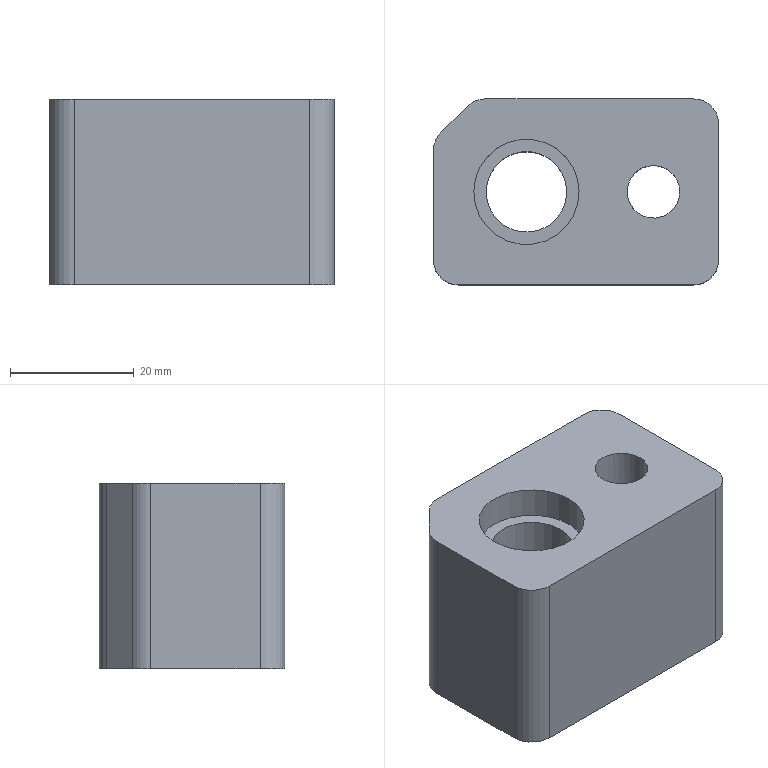Part | NX | features solid 2 | 1 solid | 18 faces | box 46 x 30 x 30 mm | volume 32628 mm3 | plane 9 | cylinder 9 | commonest cylinder face diameters 8 x5 8.5 x1 13 x1 14.5 x1 17 x1
STEP:
#1=CARTESIAN_POINT('',(3382.938,-41.938,91.));
#2=VERTEX_POINT('',#1);
#3=CARTESIAN_POINT('',(3374.438,-41.938,91.));
#4=DIRECTION('',(0.,0.,1.));
#5=DIRECTION('',(1.,0.,0.));
#6=AXIS2_PLACEMENT_3D('',#3,#4,#5);
#7=CIRCLE('',#6,8.5);
#8=EDGE_CURVE('',#2,#2,#7,.T.);
#9=ORIENTED_EDGE('',*,*,#8,.F.);
#10=EDGE_LOOP('',(#9));
#11=FACE_BOUND('',#10,.T.);
#12=CARTESIAN_POINT('',(3363.438,-56.938,91.));
#13=VERTEX_POINT('',#12);
#14=CARTESIAN_POINT('',(3401.438,-56.938,91.));
#15=VERTEX_POINT('',#14);
#16=CARTESIAN_POINT('',(3374.438,-56.938,91.));
#17=DIRECTION('',(1.,0.,0.));
#18=VECTOR('',#17,1000.);
#19=LINE('',#16,#18);
#20=EDGE_CURVE('',#13,#15,#19,.T.);
#21=ORIENTED_EDGE('',*,*,#20,.T.);
#22=CARTESIAN_POINT('',(3405.438,-52.938,91.));
#23=VERTEX_POINT('',#22);
#24=CARTESIAN_POINT('',(3401.438,-52.938,91.));
#25=DIRECTION('',(0.,0.,-1.));
#26=DIRECTION('',(0.,1.,0.));
#27=AXIS2_PLACEMENT_3D('',#24,#25,#26);
#28=CIRCLE('',#27,4.);
#29=EDGE_CURVE('',#23,#15,#28,.T.);
#30=ORIENTED_EDGE('',*,*,#29,.F.);
#31=CARTESIAN_POINT('',(3405.438,-30.938,91.));
#32=VERTEX_POINT('',#31);
#33=CARTESIAN_POINT('',(3405.438,-41.938,91.));
#34=DIRECTION('',(0.,1.,0.));
#35=VECTOR('',#34,1000.);
#36=LINE('',#33,#35);
#37=EDGE_CURVE('',#23,#32,#36,.T.);
#38=ORIENTED_EDGE('',*,*,#37,.T.);
#39=CARTESIAN_POINT('',(3401.438,-26.938,91.));
#40=VERTEX_POINT('',#39);
#41=CARTESIAN_POINT('',(3401.438,-30.938,91.));
#42=DIRECTION('',(0.,0.,-1.));
#43=DIRECTION('',(0.,1.,0.));
#44=AXIS2_PLACEMENT_3D('',#41,#42,#43);
#45=CIRCLE('',#44,4.);
#46=EDGE_CURVE('',#40,#32,#45,.T.);
#47=ORIENTED_EDGE('',*,*,#46,.F.);
#48=CARTESIAN_POINT('',(3367.731,-26.938,91.));
#49=VERTEX_POINT('',#48);
#50=CARTESIAN_POINT('',(3374.438,-26.938,91.));
#51=DIRECTION('',(-1.,0.,0.));
#52=VECTOR('',#51,1000.);
#53=LINE('',#50,#52);
#54=EDGE_CURVE('',#40,#49,#53,.T.);
#55=ORIENTED_EDGE('',*,*,#54,.T.);
#56=CARTESIAN_POINT('',(3364.902,-28.11,91.));
#57=VERTEX_POINT('',#56);
#58=CARTESIAN_POINT('',(3367.731,-30.938,91.));
#59=DIRECTION('',(0.,0.,-1.));
#60=DIRECTION('',(0.,1.,0.));
#61=AXIS2_PLACEMENT_3D('',#58,#59,#60);
#62=CIRCLE('',#61,4.);
#63=EDGE_CURVE('',#57,#49,#62,.T.);
#64=ORIENTED_EDGE('',*,*,#63,.F.);
#65=CARTESIAN_POINT('',(3360.609,-32.403,91.));
#66=VERTEX_POINT('',#65);
#67=CARTESIAN_POINT('',(3364.006,-29.006,91.));
#68=DIRECTION('',(0.7071,0.7071,0.));
#69=VECTOR('',#68,1000.);
#70=LINE('',#67,#69);
#71=EDGE_CURVE('',#66,#57,#70,.T.);
#72=ORIENTED_EDGE('',*,*,#71,.F.);
#73=CARTESIAN_POINT('',(3359.438,-35.231,91.));
#74=VERTEX_POINT('',#73);
#75=CARTESIAN_POINT('',(3363.438,-35.231,91.));
#76=DIRECTION('',(0.,0.,-1.));
#77=DIRECTION('',(0.,1.,0.));
#78=AXIS2_PLACEMENT_3D('',#75,#76,#77);
#79=CIRCLE('',#78,4.);
#80=EDGE_CURVE('',#74,#66,#79,.T.);
#81=ORIENTED_EDGE('',*,*,#80,.F.);
#82=CARTESIAN_POINT('',(3359.438,-52.938,91.));
#83=VERTEX_POINT('',#82);
#84=CARTESIAN_POINT('',(3359.438,-41.938,91.));
#85=DIRECTION('',(0.,-1.,0.));
#86=VECTOR('',#85,1000.);
#87=LINE('',#84,#86);
#88=EDGE_CURVE('',#74,#83,#87,.T.);
#89=ORIENTED_EDGE('',*,*,#88,.T.);
#90=CARTESIAN_POINT('',(3363.438,-52.938,91.));
#91=DIRECTION('',(0.,0.,-1.));
#92=DIRECTION('',(0.,1.,0.));
#93=AXIS2_PLACEMENT_3D('',#90,#91,#92);
#94=CIRCLE('',#93,4.);
#95=EDGE_CURVE('',#13,#83,#94,.T.);
#96=ORIENTED_EDGE('',*,*,#95,.F.);
#97=EDGE_LOOP('',(#21,#30,#38,#47,#55,#64,#72,#81,#89,#96));
#98=FACE_BOUND('',#97,.T.);
#99=CARTESIAN_POINT('',(3394.938,-37.688,91.));
#100=VERTEX_POINT('',#99);
#101=CARTESIAN_POINT('',(3394.938,-41.938,91.));
#102=DIRECTION('',(0.,0.,1.));
#103=DIRECTION('',(0.,1.,0.));
#104=AXIS2_PLACEMENT_3D('',#101,#102,#103);
#105=CIRCLE('',#104,4.25);
#106=EDGE_CURVE('',#100,#100,#105,.T.);
#107=ORIENTED_EDGE('',*,*,#106,.F.);
#108=EDGE_LOOP('',(#107));
#109=FACE_BOUND('',#108,.T.);
#110=CARTESIAN_POINT('',(3376.938,-41.938,91.));
#111=DIRECTION('',(0.,0.,1.));
#112=DIRECTION('',(0.,-1.,0.));
#113=AXIS2_PLACEMENT_3D('',#110,#111,#112);
#114=PLANE('',#113);
#115=ADVANCED_FACE('',(#11,#98,#109),#114,.T.);
#116=CARTESIAN_POINT('',(3367.938,-41.938,61.));
#117=VERTEX_POINT('',#116);
#118=CARTESIAN_POINT('',(3374.438,-41.938,61.));
#119=DIRECTION('',(0.,0.,-1.));
#120=DIRECTION('',(-1.,0.,0.));
#121=AXIS2_PLACEMENT_3D('',#118,#119,#120);
#122=CIRCLE('',#121,6.5);
#123=EDGE_CURVE('',#117,#117,#122,.T.);
#124=ORIENTED_EDGE('',*,*,#123,.F.);
#125=EDGE_LOOP('',(#124));
#126=FACE_BOUND('',#125,.T.);
#127=CARTESIAN_POINT('',(3387.688,-41.938,61.));
#128=VERTEX_POINT('',#127);
#129=CARTESIAN_POINT('',(3394.938,-41.938,61.));
#130=DIRECTION('',(0.,0.,1.));
#131=DIRECTION('',(-1.,0.,0.));
#132=AXIS2_PLACEMENT_3D('',#129,#130,#131);
#133=CIRCLE('',#132,7.25);
#134=EDGE_CURVE('',#128,#128,#133,.T.);
#135=ORIENTED_EDGE('',*,*,#134,.T.);
#136=EDGE_LOOP('',(#135));
#137=FACE_BOUND('',#136,.T.);
#138=CARTESIAN_POINT('',(3405.438,-30.938,61.));
#139=VERTEX_POINT('',#138);
#140=CARTESIAN_POINT('',(3405.438,-52.938,61.));
#141=VERTEX_POINT('',#140);
#142=CARTESIAN_POINT('',(3405.438,135.062,61.));
#143=DIRECTION('',(0.,-1.,0.));
#144=VECTOR('',#143,1000.);
#145=LINE('',#142,#144);
#146=EDGE_CURVE('',#139,#141,#145,.T.);
#147=ORIENTED_EDGE('',*,*,#146,.T.);
#148=CARTESIAN_POINT('',(3401.438,-56.938,61.));
#149=VERTEX_POINT('',#148);
#150=CARTESIAN_POINT('',(3401.438,-52.938,61.));
#151=DIRECTION('',(0.,0.,1.));
#152=DIRECTION('',(-1.,0.,0.));
#153=AXIS2_PLACEMENT_3D('',#150,#151,#152);
#154=CIRCLE('',#153,4.);
#155=EDGE_CURVE('',#149,#141,#154,.T.);
#156=ORIENTED_EDGE('',*,*,#155,.F.);
#157=CARTESIAN_POINT('',(3363.438,-56.938,61.));
#158=VERTEX_POINT('',#157);
#159=CARTESIAN_POINT('',(3371.438,-56.938,61.));
#160=DIRECTION('',(-1.,0.,0.));
#161=VECTOR('',#160,1000.);
#162=LINE('',#159,#161);
#163=EDGE_CURVE('',#149,#158,#162,.T.);
#164=ORIENTED_EDGE('',*,*,#163,.T.);
#165=CARTESIAN_POINT('',(3359.438,-52.938,61.));
#166=VERTEX_POINT('',#165);
#167=CARTESIAN_POINT('',(3363.438,-52.938,61.));
#168=DIRECTION('',(0.,0.,1.));
#169=DIRECTION('',(-1.,0.,0.));
#170=AXIS2_PLACEMENT_3D('',#167,#168,#169);
#171=CIRCLE('',#170,4.);
#172=EDGE_CURVE('',#166,#158,#171,.T.);
#173=ORIENTED_EDGE('',*,*,#172,.F.);
#174=CARTESIAN_POINT('',(3359.438,-35.231,61.));
#175=VERTEX_POINT('',#174);
#176=CARTESIAN_POINT('',(3359.438,135.062,61.));
#177=DIRECTION('',(0.,1.,0.));
#178=VECTOR('',#177,1000.);
#179=LINE('',#176,#178);
#180=EDGE_CURVE('',#166,#175,#179,.T.);
#181=ORIENTED_EDGE('',*,*,#180,.T.);
#182=CARTESIAN_POINT('',(3360.609,-32.403,61.));
#183=VERTEX_POINT('',#182);
#184=CARTESIAN_POINT('',(3363.438,-35.231,61.));
#185=DIRECTION('',(0.,0.,1.));
#186=DIRECTION('',(-1.,0.,0.));
#187=AXIS2_PLACEMENT_3D('',#184,#185,#186);
#188=CIRCLE('',#187,4.);
#189=EDGE_CURVE('',#183,#175,#188,.T.);
#190=ORIENTED_EDGE('',*,*,#189,.F.);
#191=CARTESIAN_POINT('',(3364.902,-28.11,61.));
#192=VERTEX_POINT('',#191);
#193=CARTESIAN_POINT('',(3449.756,56.744,61.));
#194=DIRECTION('',(-0.7071,-0.7071,0.));
#195=VECTOR('',#194,1000.);
#196=LINE('',#193,#195);
#197=EDGE_CURVE('',#192,#183,#196,.T.);
#198=ORIENTED_EDGE('',*,*,#197,.F.);
#199=CARTESIAN_POINT('',(3367.731,-26.938,61.));
#200=VERTEX_POINT('',#199);
#201=CARTESIAN_POINT('',(3367.731,-30.938,61.));
#202=DIRECTION('',(0.,0.,1.));
#203=DIRECTION('',(-1.,0.,0.));
#204=AXIS2_PLACEMENT_3D('',#201,#202,#203);
#205=CIRCLE('',#204,4.);
#206=EDGE_CURVE('',#200,#192,#205,.T.);
#207=ORIENTED_EDGE('',*,*,#206,.F.);
#208=CARTESIAN_POINT('',(3401.438,-26.938,61.));
#209=VERTEX_POINT('',#208);
#210=CARTESIAN_POINT('',(3371.438,-26.938,61.));
#211=DIRECTION('',(1.,0.,0.));
#212=VECTOR('',#211,1000.);
#213=LINE('',#210,#212);
#214=EDGE_CURVE('',#200,#209,#213,.T.);
#215=ORIENTED_EDGE('',*,*,#214,.T.);
#216=CARTESIAN_POINT('',(3401.438,-30.938,61.));
#217=DIRECTION('',(0.,0.,1.));
#218=DIRECTION('',(-1.,0.,0.));
#219=AXIS2_PLACEMENT_3D('',#216,#217,#218);
#220=CIRCLE('',#219,4.);
#221=EDGE_CURVE('',#139,#209,#220,.T.);
#222=ORIENTED_EDGE('',*,*,#221,.F.);
#223=EDGE_LOOP('',(#147,#156,#164,#173,#181,#190,#198,#207,#215,#222));
#224=FACE_BOUND('',#223,.T.);
#225=CARTESIAN_POINT('',(3371.438,135.062,61.));
#226=DIRECTION('',(0.,0.,-1.));
#227=DIRECTION('',(0.,-1.,0.));
#228=AXIS2_PLACEMENT_3D('',#225,#226,#227);
#229=PLANE('',#228);
#230=ADVANCED_FACE('',(#126,#137,#224),#229,.T.);
#231=ORIENTED_EDGE('',*,*,#88,.F.);
#232=CARTESIAN_POINT('',(3359.438,-35.231,-5.));
#233=DIRECTION('',(0.,0.,1.));
#234=VECTOR('',#233,1000.);
#235=LINE('',#232,#234);
#236=EDGE_CURVE('',#175,#74,#235,.T.);
#237=ORIENTED_EDGE('',*,*,#236,.F.);
#238=ORIENTED_EDGE('',*,*,#180,.F.);
#239=CARTESIAN_POINT('',(3359.438,-52.938,-5.));
#240=DIRECTION('',(0.,0.,-1.));
#241=VECTOR('',#240,1000.);
#242=LINE('',#239,#241);
#243=EDGE_CURVE('',#83,#166,#242,.T.);
#244=ORIENTED_EDGE('',*,*,#243,.F.);
#245=EDGE_LOOP('',(#231,#237,#238,#244));
#246=FACE_BOUND('',#245,.T.);
#247=CARTESIAN_POINT('',(3359.438,-41.938,-5.));
#248=DIRECTION('',(-1.,0.,0.));
#249=DIRECTION('',(0.,0.,-1.));
#250=AXIS2_PLACEMENT_3D('',#247,#248,#249);
#251=PLANE('',#250);
#252=ADVANCED_FACE('',(#246),#251,.T.);
#253=ORIENTED_EDGE('',*,*,#54,.F.);
#254=CARTESIAN_POINT('',(3401.438,-26.938,-5.));
#255=DIRECTION('',(0.,0.,1.));
#256=VECTOR('',#255,1000.);
#257=LINE('',#254,#256);
#258=EDGE_CURVE('',#209,#40,#257,.T.);
#259=ORIENTED_EDGE('',*,*,#258,.F.);
#260=ORIENTED_EDGE('',*,*,#214,.F.);
#261=CARTESIAN_POINT('',(3367.731,-26.938,-5.));
#262=DIRECTION('',(0.,0.,-1.));
#263=VECTOR('',#262,1000.);
#264=LINE('',#261,#263);
#265=EDGE_CURVE('',#49,#200,#264,.T.);
#266=ORIENTED_EDGE('',*,*,#265,.F.);
#267=EDGE_LOOP('',(#253,#259,#260,#266));
#268=FACE_BOUND('',#267,.T.);
#269=CARTESIAN_POINT('',(3374.438,-26.938,-5.));
#270=DIRECTION('',(0.,1.,0.));
#271=DIRECTION('',(0.,0.,1.));
#272=AXIS2_PLACEMENT_3D('',#269,#270,#271);
#273=PLANE('',#272);
#274=ADVANCED_FACE('',(#268),#273,.T.);
#275=ORIENTED_EDGE('',*,*,#37,.F.);
#276=CARTESIAN_POINT('',(3405.438,-52.938,-5.));
#277=DIRECTION('',(0.,0.,1.));
#278=VECTOR('',#277,1000.);
#279=LINE('',#276,#278);
#280=EDGE_CURVE('',#141,#23,#279,.T.);
#281=ORIENTED_EDGE('',*,*,#280,.F.);
#282=ORIENTED_EDGE('',*,*,#146,.F.);
#283=CARTESIAN_POINT('',(3405.438,-30.938,-5.));
#284=DIRECTION('',(0.,0.,-1.));
#285=VECTOR('',#284,1000.);
#286=LINE('',#283,#285);
#287=EDGE_CURVE('',#32,#139,#286,.T.);
#288=ORIENTED_EDGE('',*,*,#287,.F.);
#289=EDGE_LOOP('',(#275,#281,#282,#288));
#290=FACE_BOUND('',#289,.T.);
#291=CARTESIAN_POINT('',(3405.438,-41.938,-5.));
#292=DIRECTION('',(1.,0.,0.));
#293=DIRECTION('',(0.,0.,1.));
#294=AXIS2_PLACEMENT_3D('',#291,#292,#293);
#295=PLANE('',#294);
#296=ADVANCED_FACE('',(#290),#295,.T.);
#297=ORIENTED_EDGE('',*,*,#163,.F.);
#298=CARTESIAN_POINT('',(3401.438,-56.938,-5.));
#299=DIRECTION('',(0.,0.,-1.));
#300=VECTOR('',#299,1000.);
#301=LINE('',#298,#300);
#302=EDGE_CURVE('',#15,#149,#301,.T.);
#303=ORIENTED_EDGE('',*,*,#302,.F.);
#304=ORIENTED_EDGE('',*,*,#20,.F.);
#305=CARTESIAN_POINT('',(3363.438,-56.938,-5.));
#306=DIRECTION('',(0.,0.,1.));
#307=VECTOR('',#306,1000.);
#308=LINE('',#305,#307);
#309=EDGE_CURVE('',#158,#13,#308,.T.);
#310=ORIENTED_EDGE('',*,*,#309,.F.);
#311=EDGE_LOOP('',(#297,#303,#304,#310));
#312=FACE_BOUND('',#311,.T.);
#313=CARTESIAN_POINT('',(3374.438,-56.938,-5.));
#314=DIRECTION('',(0.,-1.,0.));
#315=DIRECTION('',(0.,0.,-1.));
#316=AXIS2_PLACEMENT_3D('',#313,#314,#315);
#317=PLANE('',#316);
#318=ADVANCED_FACE('',(#312),#317,.T.);
#319=ORIENTED_EDGE('',*,*,#71,.T.);
#320=CARTESIAN_POINT('',(3364.902,-28.11,-5.));
#321=DIRECTION('',(0.,0.,1.));
#322=VECTOR('',#321,1000.);
#323=LINE('',#320,#322);
#324=EDGE_CURVE('',#192,#57,#323,.T.);
#325=ORIENTED_EDGE('',*,*,#324,.F.);
#326=ORIENTED_EDGE('',*,*,#197,.T.);
#327=CARTESIAN_POINT('',(3360.609,-32.403,-5.));
#328=DIRECTION('',(0.,0.,-1.));
#329=VECTOR('',#328,1000.);
#330=LINE('',#327,#329);
#331=EDGE_CURVE('',#66,#183,#330,.T.);
#332=ORIENTED_EDGE('',*,*,#331,.F.);
#333=EDGE_LOOP('',(#319,#325,#326,#332));
#334=FACE_BOUND('',#333,.T.);
#335=CARTESIAN_POINT('',(3366.756,-26.256,-5.));
#336=DIRECTION('',(0.7071,-0.7071,0.));
#337=DIRECTION('',(0.,0.,1.));
#338=AXIS2_PLACEMENT_3D('',#335,#336,#337);
#339=PLANE('',#338);
#340=ADVANCED_FACE('',(#334),#339,.F.);
#341=ORIENTED_EDGE('',*,*,#155,.T.);
#342=ORIENTED_EDGE('',*,*,#280,.T.);
#343=ORIENTED_EDGE('',*,*,#29,.T.);
#344=ORIENTED_EDGE('',*,*,#302,.T.);
#345=EDGE_LOOP('',(#341,#342,#343,#344));
#346=FACE_BOUND('',#345,.T.);
#347=CARTESIAN_POINT('',(3401.438,-52.938,-5.));
#348=DIRECTION('',(0.,0.,-1.));
#349=DIRECTION('',(0.,-1.,0.));
#350=AXIS2_PLACEMENT_3D('',#347,#348,#349);
#351=CYLINDRICAL_SURFACE('',#350,4.);
#352=ADVANCED_FACE('',(#346),#351,.T.);
#353=ORIENTED_EDGE('',*,*,#221,.T.);
#354=ORIENTED_EDGE('',*,*,#258,.T.);
#355=ORIENTED_EDGE('',*,*,#46,.T.);
#356=ORIENTED_EDGE('',*,*,#287,.T.);
#357=EDGE_LOOP('',(#353,#354,#355,#356));
#358=FACE_BOUND('',#357,.T.);
#359=CARTESIAN_POINT('',(3401.438,-30.938,-5.));
#360=DIRECTION('',(0.,0.,-1.));
#361=DIRECTION('',(0.,-1.,0.));
#362=AXIS2_PLACEMENT_3D('',#359,#360,#361);
#363=CYLINDRICAL_SURFACE('',#362,4.);
#364=ADVANCED_FACE('',(#358),#363,.T.);
#365=ORIENTED_EDGE('',*,*,#206,.T.);
#366=ORIENTED_EDGE('',*,*,#324,.T.);
#367=ORIENTED_EDGE('',*,*,#63,.T.);
#368=ORIENTED_EDGE('',*,*,#265,.T.);
#369=EDGE_LOOP('',(#365,#366,#367,#368));
#370=FACE_BOUND('',#369,.T.);
#371=CARTESIAN_POINT('',(3367.731,-30.938,-5.));
#372=DIRECTION('',(0.,0.,1.));
#373=DIRECTION('',(0.,1.,0.));
#374=AXIS2_PLACEMENT_3D('',#371,#372,#373);
#375=CYLINDRICAL_SURFACE('',#374,4.);
#376=ADVANCED_FACE('',(#370),#375,.T.);
#377=ORIENTED_EDGE('',*,*,#80,.T.);
#378=ORIENTED_EDGE('',*,*,#331,.T.);
#379=ORIENTED_EDGE('',*,*,#189,.T.);
#380=ORIENTED_EDGE('',*,*,#236,.T.);
#381=EDGE_LOOP('',(#377,#378,#379,#380));
#382=FACE_BOUND('',#381,.T.);
#383=CARTESIAN_POINT('',(3363.438,-35.231,-5.));
#384=DIRECTION('',(0.,0.,-1.));
#385=DIRECTION('',(0.,-1.,0.));
#386=AXIS2_PLACEMENT_3D('',#383,#384,#385);
#387=CYLINDRICAL_SURFACE('',#386,4.);
#388=ADVANCED_FACE('',(#382),#387,.T.);
#389=ORIENTED_EDGE('',*,*,#172,.T.);
#390=ORIENTED_EDGE('',*,*,#309,.T.);
#391=ORIENTED_EDGE('',*,*,#95,.T.);
#392=ORIENTED_EDGE('',*,*,#243,.T.);
#393=EDGE_LOOP('',(#389,#390,#391,#392));
#394=FACE_BOUND('',#393,.T.);
#395=CARTESIAN_POINT('',(3363.438,-52.938,-5.));
#396=DIRECTION('',(0.,0.,-1.));
#397=DIRECTION('',(0.,-1.,0.));
#398=AXIS2_PLACEMENT_3D('',#395,#396,#397);
#399=CYLINDRICAL_SURFACE('',#398,4.);
#400=ADVANCED_FACE('',(#394),#399,.T.);
#401=CARTESIAN_POINT('',(3399.188,-41.938,76.));
#402=VERTEX_POINT('',#401);
#403=CARTESIAN_POINT('',(3394.938,-41.938,76.));
#404=DIRECTION('',(0.,0.,-1.));
#405=DIRECTION('',(1.,0.,0.));
#406=AXIS2_PLACEMENT_3D('',#403,#404,#405);
#407=CIRCLE('',#406,4.25);
#408=EDGE_CURVE('',#402,#402,#407,.T.);
#409=ORIENTED_EDGE('',*,*,#408,.T.);
#410=EDGE_LOOP('',(#409));
#411=FACE_BOUND('',#410,.T.);
#412=ORIENTED_EDGE('',*,*,#106,.T.);
#413=EDGE_LOOP('',(#412));
#414=FACE_BOUND('',#413,.T.);
#415=CARTESIAN_POINT('',(3394.938,-41.938,55.));
#416=DIRECTION('',(0.,0.,1.));
#417=DIRECTION('',(0.,-1.,0.));
#418=AXIS2_PLACEMENT_3D('',#415,#416,#417);
#419=CYLINDRICAL_SURFACE('',#418,4.25);
#420=ADVANCED_FACE('',(#411,#414),#419,.F.);
#421=ORIENTED_EDGE('',*,*,#408,.F.);
#422=EDGE_LOOP('',(#421));
#423=FACE_BOUND('',#422,.T.);
#424=CARTESIAN_POINT('',(3402.188,-41.938,76.));
#425=VERTEX_POINT('',#424);
#426=CARTESIAN_POINT('',(3394.938,-41.938,76.));
#427=DIRECTION('',(0.,0.,-1.));
#428=DIRECTION('',(1.,0.,0.));
#429=AXIS2_PLACEMENT_3D('',#426,#427,#428);
#430=CIRCLE('',#429,7.25);
#431=EDGE_CURVE('',#425,#425,#430,.T.);
#432=ORIENTED_EDGE('',*,*,#431,.T.);
#433=EDGE_LOOP('',(#432));
#434=FACE_BOUND('',#433,.T.);
#435=CARTESIAN_POINT('',(3207.938,-41.938,76.));
#436=DIRECTION('',(0.,0.,1.));
#437=DIRECTION('',(0.,-1.,0.));
#438=AXIS2_PLACEMENT_3D('',#435,#436,#437);
#439=PLANE('',#438);
#440=ADVANCED_FACE('',(#423,#434),#439,.F.);
#441=ORIENTED_EDGE('',*,*,#134,.F.);
#442=EDGE_LOOP('',(#441));
#443=FACE_BOUND('',#442,.T.);
#444=ORIENTED_EDGE('',*,*,#431,.F.);
#445=EDGE_LOOP('',(#444));
#446=FACE_BOUND('',#445,.T.);
#447=CARTESIAN_POINT('',(3394.938,-41.938,55.));
#448=DIRECTION('',(0.,0.,1.));
#449=DIRECTION('',(0.,-1.,0.));
#450=AXIS2_PLACEMENT_3D('',#447,#448,#449);
#451=CYLINDRICAL_SURFACE('',#450,7.25);
#452=ADVANCED_FACE('',(#443,#446),#451,.F.);
#453=ORIENTED_EDGE('',*,*,#123,.T.);
#454=EDGE_LOOP('',(#453));
#455=FACE_BOUND('',#454,.T.);
#456=CARTESIAN_POINT('',(3367.938,-41.938,86.));
#457=VERTEX_POINT('',#456);
#458=CARTESIAN_POINT('',(3374.438,-41.938,86.));
#459=DIRECTION('',(0.,0.,-1.));
#460=DIRECTION('',(-1.,0.,0.));
#461=AXIS2_PLACEMENT_3D('',#458,#459,#460);
#462=CIRCLE('',#461,6.5);
#463=EDGE_CURVE('',#457,#457,#462,.T.);
#464=ORIENTED_EDGE('',*,*,#463,.F.);
#465=EDGE_LOOP('',(#464));
#466=FACE_BOUND('',#465,.T.);
#467=CARTESIAN_POINT('',(3374.438,-41.938,86.));
#468=DIRECTION('',(0.,0.,-1.));
#469=DIRECTION('',(1.,0.,0.));
#470=AXIS2_PLACEMENT_3D('',#467,#468,#469);
#471=CYLINDRICAL_SURFACE('',#470,6.5);
#472=ADVANCED_FACE('',(#455,#466),#471,.F.);
#473=ORIENTED_EDGE('',*,*,#463,.T.);
#474=EDGE_LOOP('',(#473));
#475=FACE_BOUND('',#474,.T.);
#476=CARTESIAN_POINT('',(3365.938,-41.938,86.));
#477=VERTEX_POINT('',#476);
#478=CARTESIAN_POINT('',(3374.438,-41.938,86.));
#479=DIRECTION('',(0.,0.,-1.));
#480=DIRECTION('',(-1.,0.,0.));
#481=AXIS2_PLACEMENT_3D('',#478,#479,#480);
#482=CIRCLE('',#481,8.5);
#483=EDGE_CURVE('',#477,#477,#482,.T.);
#484=ORIENTED_EDGE('',*,*,#483,.F.);
#485=EDGE_LOOP('',(#484));
#486=FACE_BOUND('',#485,.T.);
#487=CARTESIAN_POINT('',(3374.438,-41.938,86.));
#488=DIRECTION('',(0.,0.,-1.));
#489=DIRECTION('',(0.,-1.,0.));
#490=AXIS2_PLACEMENT_3D('',#487,#488,#489);
#491=PLANE('',#490);
#492=ADVANCED_FACE('',(#475,#486),#491,.F.);
#493=ORIENTED_EDGE('',*,*,#8,.T.);
#494=EDGE_LOOP('',(#493));
#495=FACE_BOUND('',#494,.T.);
#496=ORIENTED_EDGE('',*,*,#483,.T.);
#497=EDGE_LOOP('',(#496));
#498=FACE_BOUND('',#497,.T.);
#499=CARTESIAN_POINT('',(3374.438,-41.938,88.5));
#500=DIRECTION('',(0.,0.,-1.));
#501=DIRECTION('',(-1.,0.,0.));
#502=AXIS2_PLACEMENT_3D('',#499,#500,#501);
#503=CYLINDRICAL_SURFACE('',#502,8.5);
#504=ADVANCED_FACE('',(#495,#498),#503,.F.);
#505=CLOSED_SHELL('',(#115,#230,#252,#274,#296,#318,#340,#352,#364,#376,#388,#400,#420,#440,#452,#472,#492,#504));
#506=MANIFOLD_SOLID_BREP('',#505);
#507=(LENGTH_UNIT()NAMED_UNIT(*)SI_UNIT(.MILLI.,.METRE.));
#508=UNCERTAINTY_MEASURE_WITH_UNIT(LENGTH_MEASURE(0.00001),#507,'','');
#509=(NAMED_UNIT(*)PLANE_ANGLE_UNIT()SI_UNIT($,.RADIAN.));
#510=(NAMED_UNIT(*)SI_UNIT($,.STERADIAN.)SOLID_ANGLE_UNIT());
#511=(GEOMETRIC_REPRESENTATION_CONTEXT(3)GLOBAL_UNCERTAINTY_ASSIGNED_CONTEXT((#508))GLOBAL_UNIT_ASSIGNED_CONTEXT((#507,#509,#510))REPRESENTATION_CONTEXT('',''));
#512=ADVANCED_BREP_SHAPE_REPRESENTATION('',(#506),#511);